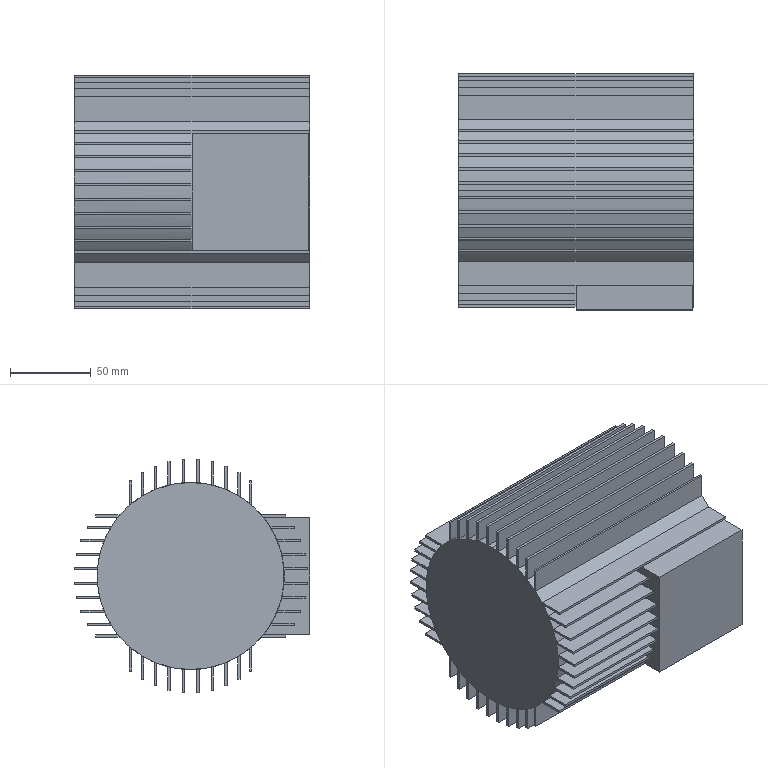Part | SolidWorks | features BaseBody 1 | 1 solid | 233 faces | box 146 x 146.326 x 144.651 mm | volume 1760693 mm3 | plane 231 | cylinder 2 | commonest cylinder face diameters 116 x2